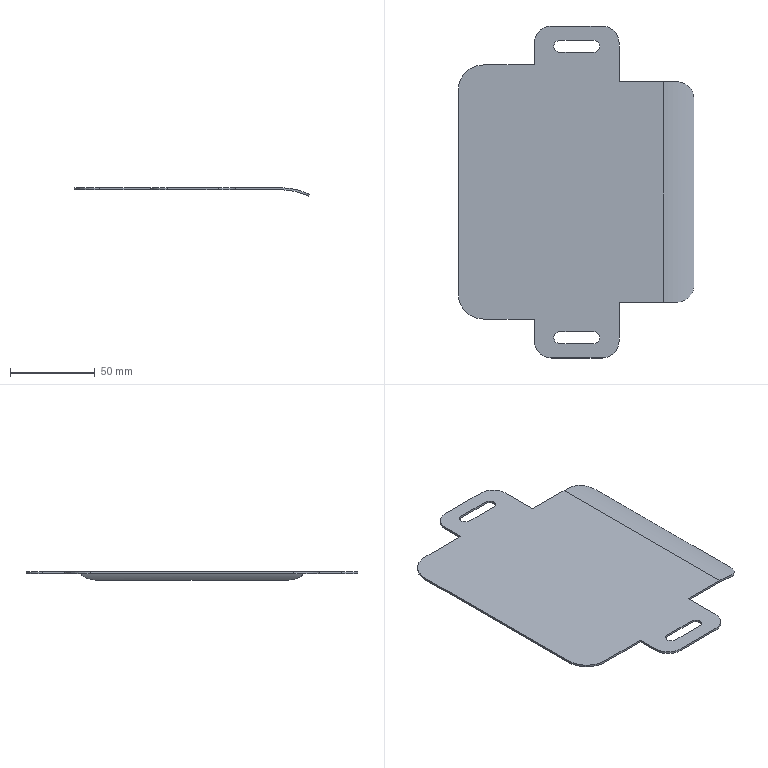Part | STEP file | YBQDJ-YB-32 | 1 solid | 32 faces | box 139.076 x 196 x 5.026 mm | volume 26086 mm3 | plane 18 | cylinder 14 | commonest cylinder face diameters 20 x6 7 x4 30 x2 83.301 x1 85.701 x1